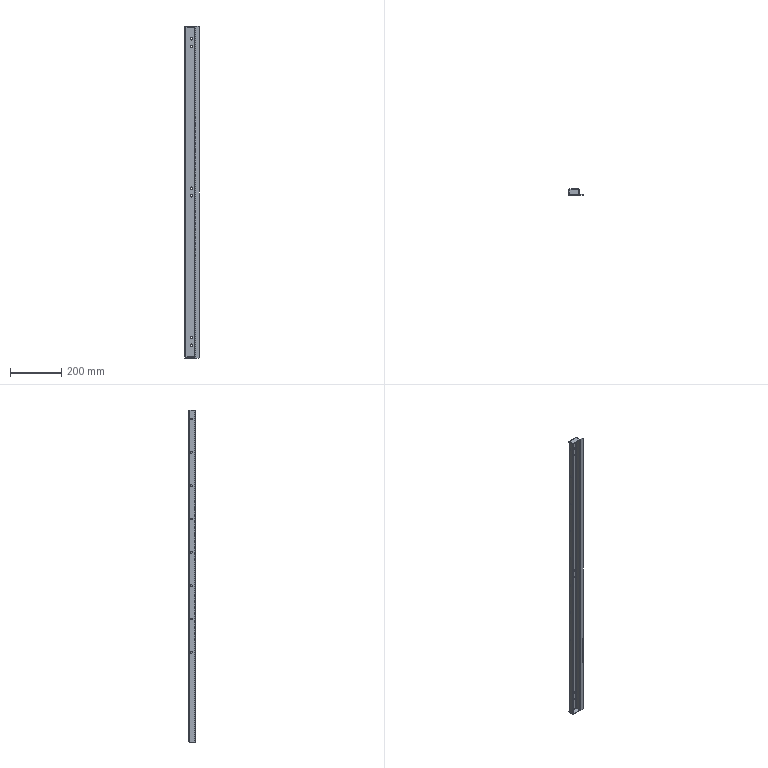Part | NX | features solid 2 | 1 solid | 80 faces | box 55 x 25 x 1295 mm | volume 248984 mm3 | plane 42 | cylinder 38 | commonest cylinder face diameters 7 x16 9.3 x12 4 x5 8 x5